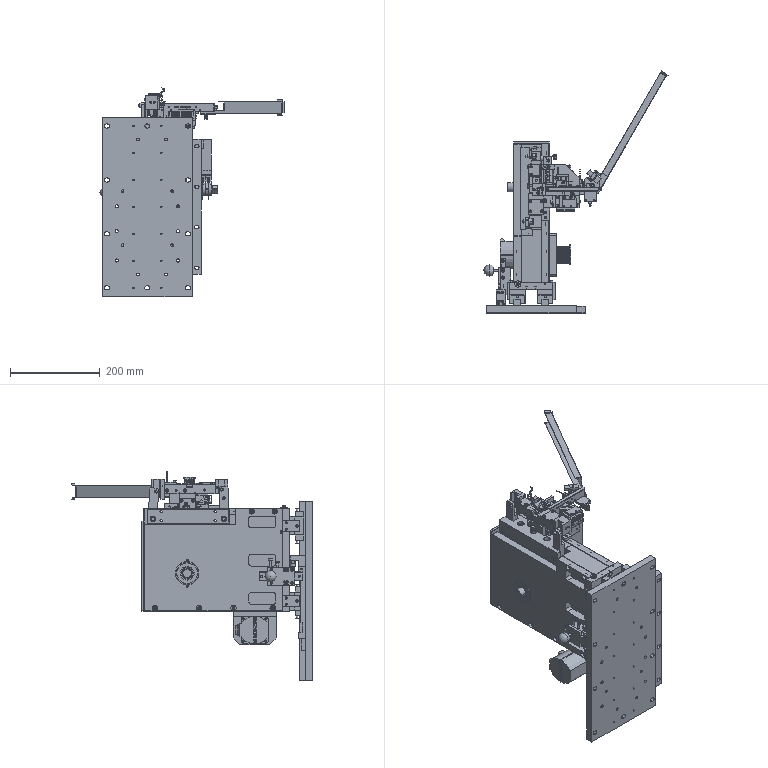Part | NX | 191 solids | 11783 faces | volume 6439488 mm3 | plane 5876 | cylinder 4215 | cone 1044 | torus 390 | spline 129 | sphere 129 | commonest cylinder face diameters 5 x557 0.5 x291 3.3 x256 0.2 x235 6.55 x176 1.1 x172